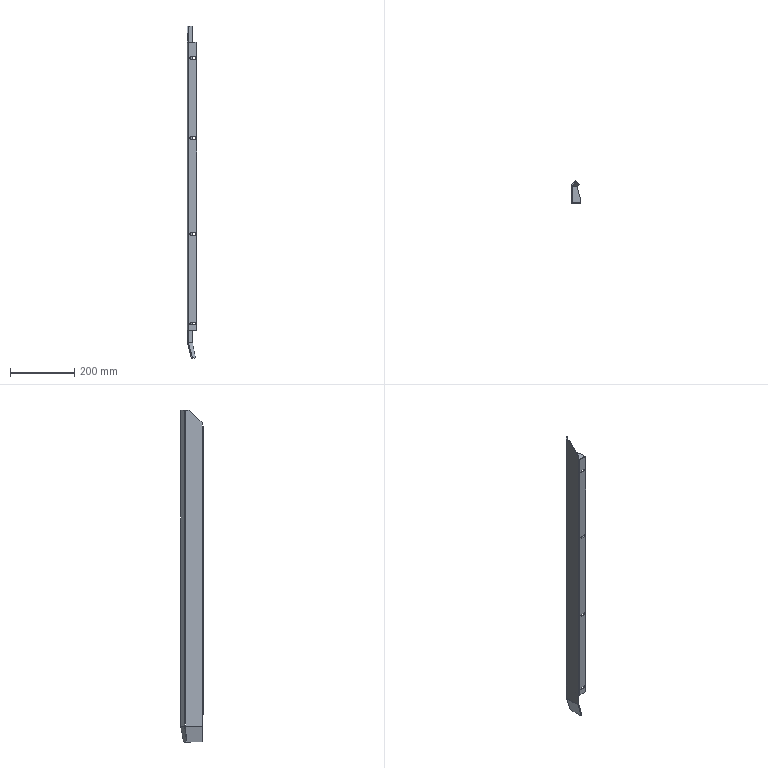Part | STEP file | Mirror Part 3 | 7 solids | 108 faces | box 30 x 71.142 x 1037 mm | volume 319137 mm3 | plane 83 | cylinder 23 | spline 2 | commonest cylinder face diameters 7 x12 5 x7 1 x4